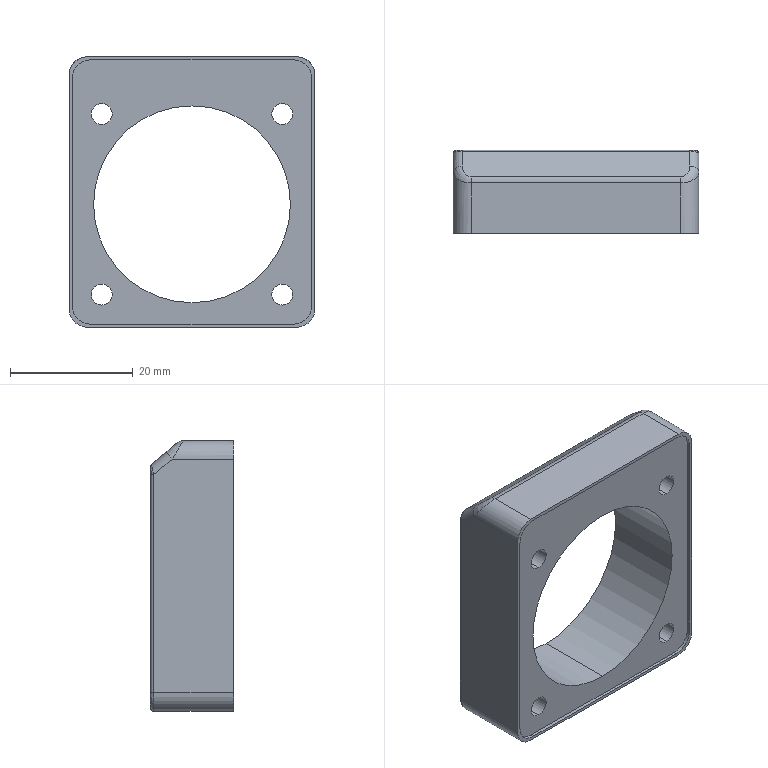Part | STEP file | 31100134--1-0001 | 1 solid | 43 faces | box 40 x 13.5 x 44 mm | volume 11515 mm3 | cylinder 25 | plane 12 | spline 6 | commonest cylinder face diameters 3.4 x8 6 x8 1 x4 3 x3 32 x2